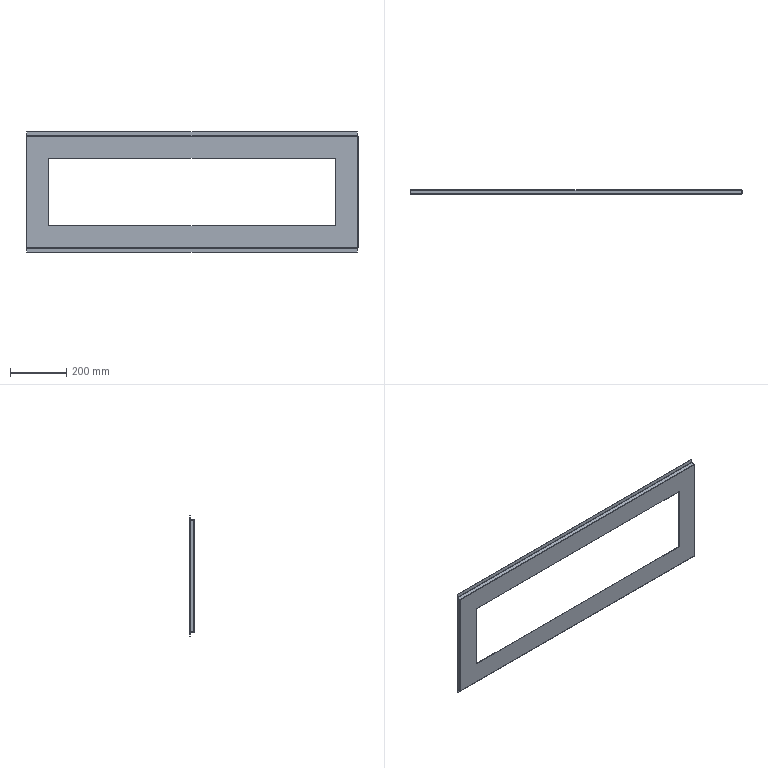Part | SolidWorks | features EdgeFlange 3, FlatPattern 1, SMBaseFlange 1, SheetMetal 1 | 1 solid | 74 faces | box 1180 x 16.2 x 427.6 mm | volume 373152 mm3 | plane 50 | cylinder 16 | spline 8 | commonest cylinder face diameters 0.9 x8 3.3 x8